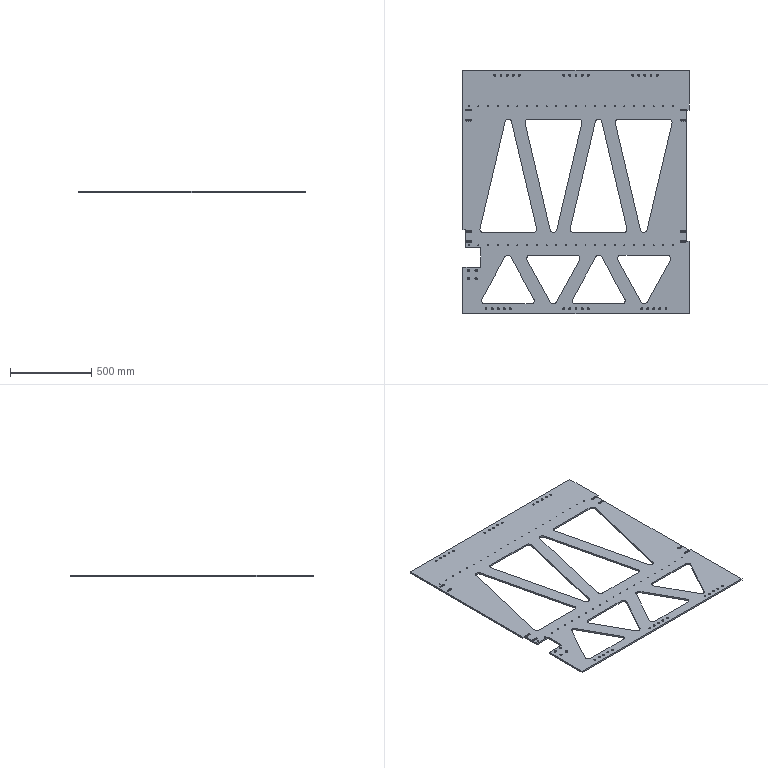Part | NX | features SIMPLE HOLE 74, SYMBOLIC_THREAD 74, DATUM_CSYS 61, SKETCH 60, EXTRACT_FACE 55, HOLE PACKAGE 55, Instance Feature 49, CBORE_HOLE 28, EXTRACT_DATUM_PLANE 7, EXTRUDE 6, Pattern Feature 6 | 1 solid | 370 faces | box 1395 x 1500 x 10 mm | volume 12886681 mm3 | cylinder 154 | cone 148 | plane 68 | commonest cylinder face diameters 5.2 x44 10.9 x30 6.5 x24 11 x24 40 x24 8.5 x4